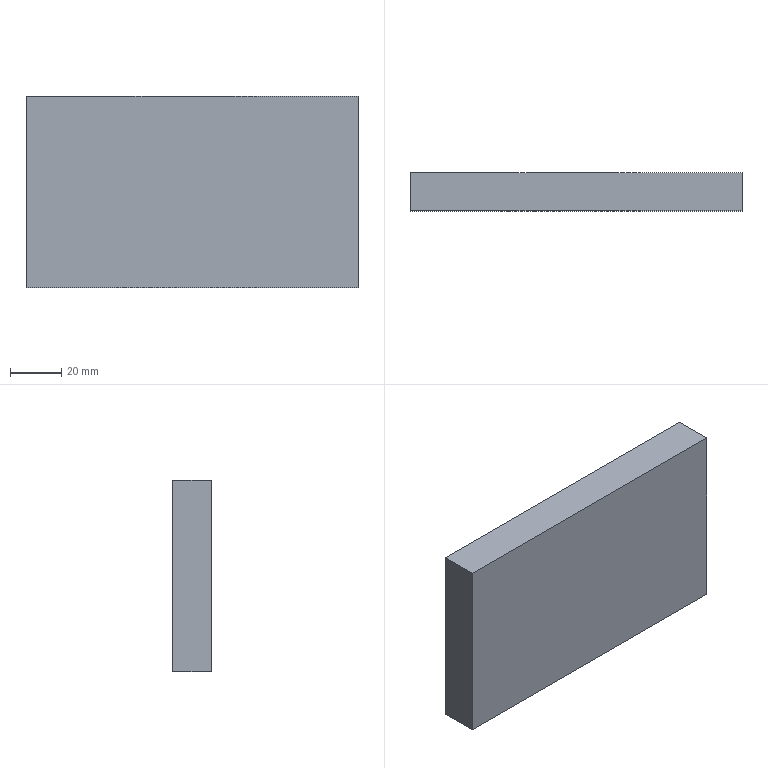Part | SolidWorks | features FlatPattern 1, SMBaseFlange 1, SheetMetal 1 | 1 solid | 6 faces | box 130 x 15 x 75 mm | volume 146250 mm3 | plane 6
STEP:
#1=CARTESIAN_POINT('',(0.,0.,0.));
#2=VERTEX_POINT('',#1);
#3=CARTESIAN_POINT('',(0.,0.,75.));
#4=VERTEX_POINT('',#3);
#5=CARTESIAN_POINT('',(0.,0.,0.));
#6=DIRECTION('',(0.,0.,1.));
#7=VECTOR('',#6,1000.);
#8=LINE('',#5,#7);
#9=EDGE_CURVE('',#2,#4,#8,.T.);
#10=ORIENTED_EDGE('',*,*,#9,.F.);
#11=CARTESIAN_POINT('',(0.,-15.,0.));
#12=VERTEX_POINT('',#11);
#13=CARTESIAN_POINT('',(0.,-15.,0.));
#14=DIRECTION('',(0.,1.,0.));
#15=VECTOR('',#14,1000.);
#16=LINE('',#13,#15);
#17=EDGE_CURVE('',#12,#2,#16,.T.);
#18=ORIENTED_EDGE('',*,*,#17,.F.);
#19=CARTESIAN_POINT('',(0.,-15.,75.));
#20=VERTEX_POINT('',#19);
#21=CARTESIAN_POINT('',(0.,-15.,0.));
#22=DIRECTION('',(0.,0.,1.));
#23=VECTOR('',#22,1000.);
#24=LINE('',#21,#23);
#25=EDGE_CURVE('',#12,#20,#24,.T.);
#26=ORIENTED_EDGE('',*,*,#25,.T.);
#27=CARTESIAN_POINT('',(0.,-15.,75.));
#28=DIRECTION('',(0.,1.,0.));
#29=VECTOR('',#28,1000.);
#30=LINE('',#27,#29);
#31=EDGE_CURVE('',#20,#4,#30,.T.);
#32=ORIENTED_EDGE('',*,*,#31,.T.);
#33=EDGE_LOOP('',(#10,#18,#26,#32));
#34=FACE_OUTER_BOUND('',#33,.T.);
#35=CARTESIAN_POINT('',(0.,-15.,0.));
#36=DIRECTION('',(-1.,0.,0.));
#37=DIRECTION('',(0.,0.,1.));
#38=AXIS2_PLACEMENT_3D('',#35,#36,#37);
#39=PLANE('',#38);
#40=ADVANCED_FACE('',(#34),#39,.T.);
#41=CARTESIAN_POINT('',(130.,0.,0.));
#42=VERTEX_POINT('',#41);
#43=CARTESIAN_POINT('',(0.,0.,0.));
#44=DIRECTION('',(-1.,0.,0.));
#45=VECTOR('',#44,1000.);
#46=LINE('',#43,#45);
#47=EDGE_CURVE('',#42,#2,#46,.T.);
#48=ORIENTED_EDGE('',*,*,#47,.F.);
#49=CARTESIAN_POINT('',(130.,-15.,0.));
#50=VERTEX_POINT('',#49);
#51=CARTESIAN_POINT('',(130.,-15.,0.));
#52=DIRECTION('',(0.,1.,0.));
#53=VECTOR('',#52,1000.);
#54=LINE('',#51,#53);
#55=EDGE_CURVE('',#50,#42,#54,.T.);
#56=ORIENTED_EDGE('',*,*,#55,.F.);
#57=CARTESIAN_POINT('',(0.,-15.,0.));
#58=DIRECTION('',(-1.,0.,0.));
#59=VECTOR('',#58,1000.);
#60=LINE('',#57,#59);
#61=EDGE_CURVE('',#50,#12,#60,.T.);
#62=ORIENTED_EDGE('',*,*,#61,.T.);
#63=ORIENTED_EDGE('',*,*,#17,.T.);
#64=EDGE_LOOP('',(#48,#56,#62,#63));
#65=FACE_OUTER_BOUND('',#64,.T.);
#66=CARTESIAN_POINT('',(0.,-15.,0.));
#67=DIRECTION('',(0.,0.,-1.));
#68=DIRECTION('',(-1.,0.,0.));
#69=AXIS2_PLACEMENT_3D('',#66,#67,#68);
#70=PLANE('',#69);
#71=ADVANCED_FACE('',(#65),#70,.T.);
#72=CARTESIAN_POINT('',(130.,0.,75.));
#73=VERTEX_POINT('',#72);
#74=CARTESIAN_POINT('',(130.,0.,0.));
#75=DIRECTION('',(0.,0.,-1.));
#76=VECTOR('',#75,1000.);
#77=LINE('',#74,#76);
#78=EDGE_CURVE('',#73,#42,#77,.T.);
#79=ORIENTED_EDGE('',*,*,#78,.F.);
#80=CARTESIAN_POINT('',(130.,-15.,75.));
#81=VERTEX_POINT('',#80);
#82=CARTESIAN_POINT('',(130.,-15.,75.));
#83=DIRECTION('',(0.,1.,0.));
#84=VECTOR('',#83,1000.);
#85=LINE('',#82,#84);
#86=EDGE_CURVE('',#81,#73,#85,.T.);
#87=ORIENTED_EDGE('',*,*,#86,.F.);
#88=CARTESIAN_POINT('',(130.,-15.,0.));
#89=DIRECTION('',(0.,0.,-1.));
#90=VECTOR('',#89,1000.);
#91=LINE('',#88,#90);
#92=EDGE_CURVE('',#81,#50,#91,.T.);
#93=ORIENTED_EDGE('',*,*,#92,.T.);
#94=ORIENTED_EDGE('',*,*,#55,.T.);
#95=EDGE_LOOP('',(#79,#87,#93,#94));
#96=FACE_OUTER_BOUND('',#95,.T.);
#97=CARTESIAN_POINT('',(130.,-15.,0.));
#98=DIRECTION('',(1.,0.,0.));
#99=DIRECTION('',(0.,0.,-1.));
#100=AXIS2_PLACEMENT_3D('',#97,#98,#99);
#101=PLANE('',#100);
#102=ADVANCED_FACE('',(#96),#101,.T.);
#103=CARTESIAN_POINT('',(0.,0.,75.));
#104=DIRECTION('',(1.,0.,0.));
#105=VECTOR('',#104,1000.);
#106=LINE('',#103,#105);
#107=EDGE_CURVE('',#4,#73,#106,.T.);
#108=ORIENTED_EDGE('',*,*,#107,.F.);
#109=ORIENTED_EDGE('',*,*,#31,.F.);
#110=CARTESIAN_POINT('',(0.,-15.,75.));
#111=DIRECTION('',(1.,0.,0.));
#112=VECTOR('',#111,1000.);
#113=LINE('',#110,#112);
#114=EDGE_CURVE('',#20,#81,#113,.T.);
#115=ORIENTED_EDGE('',*,*,#114,.T.);
#116=ORIENTED_EDGE('',*,*,#86,.T.);
#117=EDGE_LOOP('',(#108,#109,#115,#116));
#118=FACE_OUTER_BOUND('',#117,.T.);
#119=CARTESIAN_POINT('',(0.,-15.,75.));
#120=DIRECTION('',(0.,0.,1.));
#121=DIRECTION('',(1.,0.,0.));
#122=AXIS2_PLACEMENT_3D('',#119,#120,#121);
#123=PLANE('',#122);
#124=ADVANCED_FACE('',(#118),#123,.T.);
#125=ORIENTED_EDGE('',*,*,#25,.F.);
#126=ORIENTED_EDGE('',*,*,#61,.F.);
#127=ORIENTED_EDGE('',*,*,#92,.F.);
#128=ORIENTED_EDGE('',*,*,#114,.F.);
#129=EDGE_LOOP('',(#125,#126,#127,#128));
#130=FACE_OUTER_BOUND('',#129,.T.);
#131=CARTESIAN_POINT('',(0.,-15.,0.));
#132=DIRECTION('',(0.,1.,0.));
#133=DIRECTION('',(0.,0.,1.));
#134=AXIS2_PLACEMENT_3D('',#131,#132,#133);
#135=PLANE('',#134);
#136=ADVANCED_FACE('',(#130),#135,.F.);
#137=ORIENTED_EDGE('',*,*,#9,.T.);
#138=ORIENTED_EDGE('',*,*,#107,.T.);
#139=ORIENTED_EDGE('',*,*,#78,.T.);
#140=ORIENTED_EDGE('',*,*,#47,.T.);
#141=EDGE_LOOP('',(#137,#138,#139,#140));
#142=FACE_OUTER_BOUND('',#141,.T.);
#143=CARTESIAN_POINT('',(0.,0.,0.));
#144=DIRECTION('',(0.,1.,0.));
#145=DIRECTION('',(0.,0.,1.));
#146=AXIS2_PLACEMENT_3D('',#143,#144,#145);
#147=PLANE('',#146);
#148=ADVANCED_FACE('',(#142),#147,.T.);
#149=CLOSED_SHELL('',(#40,#71,#102,#124,#136,#148));
#150=MANIFOLD_SOLID_BREP('',#149);
#151=CARTESIAN_POINT('',(0.,0.,0.));
#152=DIRECTION('',(0.,0.,1.));
#153=DIRECTION('',(1.,0.,0.));
#154=AXIS2_PLACEMENT_3D('',#151,#152,#153);
#155=(LENGTH_UNIT()NAMED_UNIT(*)SI_UNIT(.MILLI.,.METRE.));
#156=UNCERTAINTY_MEASURE_WITH_UNIT(LENGTH_MEASURE(0.00001),#155,'','');
#157=(NAMED_UNIT(*)PLANE_ANGLE_UNIT()SI_UNIT($,.RADIAN.));
#158=(NAMED_UNIT(*)SI_UNIT($,.STERADIAN.)SOLID_ANGLE_UNIT());
#159=(GEOMETRIC_REPRESENTATION_CONTEXT(3)GLOBAL_UNCERTAINTY_ASSIGNED_CONTEXT((#156))GLOBAL_UNIT_ASSIGNED_CONTEXT((#155,#157,#158))REPRESENTATION_CONTEXT('',''));
#160=ADVANCED_BREP_SHAPE_REPRESENTATION('',(#150,#154),#159);